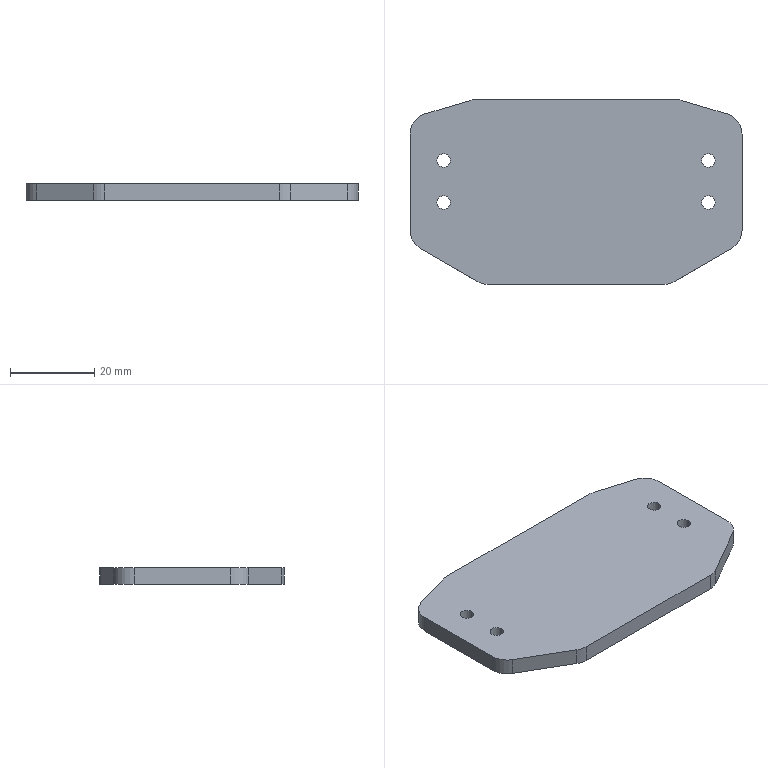Part | SolidWorks | features Extrusion 1, Fillet 1 | 1 solid | 26 faces | box 79 x 44 x 4 mm | volume 12779 mm3 | cylinder 16 | plane 10 | commonest cylinder face diameters 3.2 x8 10 x8
STEP:
#1=CARTESIAN_POINT('',(29.9,9.,4.));
#2=VERTEX_POINT('',#1);
#3=CARTESIAN_POINT('',(33.1,9.,4.));
#4=VERTEX_POINT('',#3);
#5=CARTESIAN_POINT('',(31.5,9.,4.));
#6=DIRECTION('',(0.,0.,1.));
#7=DIRECTION('',(-1.,0.,0.));
#8=AXIS2_PLACEMENT_3D('',#5,#6,#7);
#9=CIRCLE('',#8,1.6);
#10=EDGE_CURVE('',#2,#4,#9,.T.);
#11=ORIENTED_EDGE('',*,*,#10,.T.);
#12=CARTESIAN_POINT('',(33.1,9.,0.));
#13=VERTEX_POINT('',#12);
#14=CARTESIAN_POINT('',(33.1,9.,4.));
#15=DIRECTION('',(0.,0.,-1.));
#16=VECTOR('',#15,1000.);
#17=LINE('',#14,#16);
#18=EDGE_CURVE('',#4,#13,#17,.T.);
#19=ORIENTED_EDGE('',*,*,#18,.T.);
#20=CARTESIAN_POINT('',(29.9,9.,0.));
#21=VERTEX_POINT('',#20);
#22=CARTESIAN_POINT('',(31.5,9.,0.));
#23=DIRECTION('',(0.,0.,1.));
#24=DIRECTION('',(-1.,0.,0.));
#25=AXIS2_PLACEMENT_3D('',#22,#23,#24);
#26=CIRCLE('',#25,1.6);
#27=EDGE_CURVE('',#21,#13,#26,.T.);
#28=ORIENTED_EDGE('',*,*,#27,.F.);
#29=CARTESIAN_POINT('',(29.9,9.,4.));
#30=DIRECTION('',(0.,0.,-1.));
#31=VECTOR('',#30,1000.);
#32=LINE('',#29,#31);
#33=EDGE_CURVE('',#2,#21,#32,.T.);
#34=ORIENTED_EDGE('',*,*,#33,.F.);
#35=EDGE_LOOP('',(#11,#19,#28,#34));
#36=FACE_OUTER_BOUND('',#35,.T.);
#37=CARTESIAN_POINT('',(31.5,9.,4.));
#38=DIRECTION('',(0.,0.,-1.));
#39=DIRECTION('',(-1.,0.,0.));
#40=AXIS2_PLACEMENT_3D('',#37,#38,#39);
#41=CYLINDRICAL_SURFACE('',#40,1.6);
#42=ADVANCED_FACE('',(#36),#41,.F.);
#43=CARTESIAN_POINT('',(29.9,-1.,4.));
#44=VERTEX_POINT('',#43);
#45=CARTESIAN_POINT('',(33.1,-1.,4.));
#46=VERTEX_POINT('',#45);
#47=CARTESIAN_POINT('',(31.5,-1.,4.));
#48=DIRECTION('',(0.,0.,1.));
#49=DIRECTION('',(-1.,0.,0.));
#50=AXIS2_PLACEMENT_3D('',#47,#48,#49);
#51=CIRCLE('',#50,1.6);
#52=EDGE_CURVE('',#44,#46,#51,.T.);
#53=ORIENTED_EDGE('',*,*,#52,.T.);
#54=CARTESIAN_POINT('',(33.1,-1.,0.));
#55=VERTEX_POINT('',#54);
#56=CARTESIAN_POINT('',(33.1,-1.,4.));
#57=DIRECTION('',(0.,0.,-1.));
#58=VECTOR('',#57,1000.);
#59=LINE('',#56,#58);
#60=EDGE_CURVE('',#46,#55,#59,.T.);
#61=ORIENTED_EDGE('',*,*,#60,.T.);
#62=CARTESIAN_POINT('',(29.9,-1.,0.));
#63=VERTEX_POINT('',#62);
#64=CARTESIAN_POINT('',(31.5,-1.,0.));
#65=DIRECTION('',(0.,0.,1.));
#66=DIRECTION('',(-1.,0.,0.));
#67=AXIS2_PLACEMENT_3D('',#64,#65,#66);
#68=CIRCLE('',#67,1.6);
#69=EDGE_CURVE('',#63,#55,#68,.T.);
#70=ORIENTED_EDGE('',*,*,#69,.F.);
#71=CARTESIAN_POINT('',(29.9,-1.,4.));
#72=DIRECTION('',(0.,0.,-1.));
#73=VECTOR('',#72,1000.);
#74=LINE('',#71,#73);
#75=EDGE_CURVE('',#44,#63,#74,.T.);
#76=ORIENTED_EDGE('',*,*,#75,.F.);
#77=EDGE_LOOP('',(#53,#61,#70,#76));
#78=FACE_OUTER_BOUND('',#77,.T.);
#79=CARTESIAN_POINT('',(31.5,-1.,4.));
#80=DIRECTION('',(0.,0.,-1.));
#81=DIRECTION('',(-1.,0.,0.));
#82=AXIS2_PLACEMENT_3D('',#79,#80,#81);
#83=CYLINDRICAL_SURFACE('',#82,1.6);
#84=ADVANCED_FACE('',(#78),#83,.F.);
#85=CARTESIAN_POINT('',(-33.1,-1.,4.));
#86=VERTEX_POINT('',#85);
#87=CARTESIAN_POINT('',(-29.9,-1.,4.));
#88=VERTEX_POINT('',#87);
#89=CARTESIAN_POINT('',(-31.5,-1.,4.));
#90=DIRECTION('',(0.,0.,1.));
#91=DIRECTION('',(1.,0.,0.));
#92=AXIS2_PLACEMENT_3D('',#89,#90,#91);
#93=CIRCLE('',#92,1.6);
#94=EDGE_CURVE('',#86,#88,#93,.T.);
#95=ORIENTED_EDGE('',*,*,#94,.T.);
#96=CARTESIAN_POINT('',(-29.9,-1.,0.));
#97=VERTEX_POINT('',#96);
#98=CARTESIAN_POINT('',(-29.9,-1.,4.));
#99=DIRECTION('',(0.,0.,-1.));
#100=VECTOR('',#99,1000.);
#101=LINE('',#98,#100);
#102=EDGE_CURVE('',#88,#97,#101,.T.);
#103=ORIENTED_EDGE('',*,*,#102,.T.);
#104=CARTESIAN_POINT('',(-33.1,-1.,0.));
#105=VERTEX_POINT('',#104);
#106=CARTESIAN_POINT('',(-31.5,-1.,0.));
#107=DIRECTION('',(0.,0.,1.));
#108=DIRECTION('',(1.,0.,0.));
#109=AXIS2_PLACEMENT_3D('',#106,#107,#108);
#110=CIRCLE('',#109,1.6);
#111=EDGE_CURVE('',#105,#97,#110,.T.);
#112=ORIENTED_EDGE('',*,*,#111,.F.);
#113=CARTESIAN_POINT('',(-33.1,-1.,4.));
#114=DIRECTION('',(0.,0.,-1.));
#115=VECTOR('',#114,1000.);
#116=LINE('',#113,#115);
#117=EDGE_CURVE('',#86,#105,#116,.T.);
#118=ORIENTED_EDGE('',*,*,#117,.F.);
#119=EDGE_LOOP('',(#95,#103,#112,#118));
#120=FACE_OUTER_BOUND('',#119,.T.);
#121=CARTESIAN_POINT('',(-31.5,-1.,4.));
#122=DIRECTION('',(0.,0.,-1.));
#123=DIRECTION('',(-1.,0.,0.));
#124=AXIS2_PLACEMENT_3D('',#121,#122,#123);
#125=CYLINDRICAL_SURFACE('',#124,1.6);
#126=ADVANCED_FACE('',(#120),#125,.F.);
#127=CARTESIAN_POINT('',(-33.1,9.,4.));
#128=VERTEX_POINT('',#127);
#129=CARTESIAN_POINT('',(-29.9,9.,4.));
#130=VERTEX_POINT('',#129);
#131=CARTESIAN_POINT('',(-31.5,9.,4.));
#132=DIRECTION('',(0.,0.,1.));
#133=DIRECTION('',(1.,0.,0.));
#134=AXIS2_PLACEMENT_3D('',#131,#132,#133);
#135=CIRCLE('',#134,1.6);
#136=EDGE_CURVE('',#128,#130,#135,.T.);
#137=ORIENTED_EDGE('',*,*,#136,.T.);
#138=CARTESIAN_POINT('',(-29.9,9.,0.));
#139=VERTEX_POINT('',#138);
#140=CARTESIAN_POINT('',(-29.9,9.,4.));
#141=DIRECTION('',(0.,0.,-1.));
#142=VECTOR('',#141,1000.);
#143=LINE('',#140,#142);
#144=EDGE_CURVE('',#130,#139,#143,.T.);
#145=ORIENTED_EDGE('',*,*,#144,.T.);
#146=CARTESIAN_POINT('',(-33.1,9.,0.));
#147=VERTEX_POINT('',#146);
#148=CARTESIAN_POINT('',(-31.5,9.,0.));
#149=DIRECTION('',(0.,0.,1.));
#150=DIRECTION('',(1.,0.,0.));
#151=AXIS2_PLACEMENT_3D('',#148,#149,#150);
#152=CIRCLE('',#151,1.6);
#153=EDGE_CURVE('',#147,#139,#152,.T.);
#154=ORIENTED_EDGE('',*,*,#153,.F.);
#155=CARTESIAN_POINT('',(-33.1,9.,4.));
#156=DIRECTION('',(0.,0.,-1.));
#157=VECTOR('',#156,1000.);
#158=LINE('',#155,#157);
#159=EDGE_CURVE('',#128,#147,#158,.T.);
#160=ORIENTED_EDGE('',*,*,#159,.F.);
#161=EDGE_LOOP('',(#137,#145,#154,#160));
#162=FACE_OUTER_BOUND('',#161,.T.);
#163=CARTESIAN_POINT('',(-31.5,9.,4.));
#164=DIRECTION('',(0.,0.,-1.));
#165=DIRECTION('',(-1.,0.,0.));
#166=AXIS2_PLACEMENT_3D('',#163,#164,#165);
#167=CYLINDRICAL_SURFACE('',#166,1.6);
#168=ADVANCED_FACE('',(#162),#167,.F.);
#169=CARTESIAN_POINT('',(-39.5,15.28,4.));
#170=VERTEX_POINT('',#169);
#171=CARTESIAN_POINT('',(-39.5,-7.613,4.));
#172=VERTEX_POINT('',#171);
#173=CARTESIAN_POINT('',(-39.5,19.,4.));
#174=DIRECTION('',(0.,-1.,0.));
#175=VECTOR('',#174,1000.);
#176=LINE('',#173,#175);
#177=EDGE_CURVE('',#170,#172,#176,.T.);
#178=ORIENTED_EDGE('',*,*,#177,.T.);
#179=CARTESIAN_POINT('',(-37.,-11.943,4.));
#180=VERTEX_POINT('',#179);
#181=CARTESIAN_POINT('',(-34.5,-7.613,4.));
#182=DIRECTION('',(0.,0.,1.));
#183=DIRECTION('',(-1.,0.,0.));
#184=AXIS2_PLACEMENT_3D('',#181,#182,#183);
#185=CIRCLE('',#184,5.);
#186=EDGE_CURVE('',#172,#180,#185,.T.);
#187=ORIENTED_EDGE('',*,*,#186,.T.);
#188=CARTESIAN_POINT('',(-23.34,-19.83,4.));
#189=VERTEX_POINT('',#188);
#190=CARTESIAN_POINT('',(-39.5,-10.5,4.));
#191=DIRECTION('',(0.866,-0.5,0.));
#192=VECTOR('',#191,1000.);
#193=LINE('',#190,#192);
#194=EDGE_CURVE('',#180,#189,#193,.T.);
#195=ORIENTED_EDGE('',*,*,#194,.T.);
#196=CARTESIAN_POINT('',(-20.84,-20.5,4.));
#197=VERTEX_POINT('',#196);
#198=CARTESIAN_POINT('',(-20.84,-15.5,4.));
#199=DIRECTION('',(0.,0.,1.));
#200=DIRECTION('',(-1.,0.,0.));
#201=AXIS2_PLACEMENT_3D('',#198,#199,#200);
#202=CIRCLE('',#201,5.);
#203=EDGE_CURVE('',#189,#197,#202,.T.);
#204=ORIENTED_EDGE('',*,*,#203,.T.);
#205=CARTESIAN_POINT('',(20.84,-20.5,4.));
#206=VERTEX_POINT('',#205);
#207=CARTESIAN_POINT('',(-22.179,-20.5,4.));
#208=DIRECTION('',(1.,0.,0.));
#209=VECTOR('',#208,1000.);
#210=LINE('',#207,#209);
#211=EDGE_CURVE('',#197,#206,#210,.T.);
#212=ORIENTED_EDGE('',*,*,#211,.T.);
#213=CARTESIAN_POINT('',(23.34,-19.83,4.));
#214=VERTEX_POINT('',#213);
#215=CARTESIAN_POINT('',(20.84,-15.5,4.));
#216=DIRECTION('',(0.,0.,1.));
#217=DIRECTION('',(-1.,0.,0.));
#218=AXIS2_PLACEMENT_3D('',#215,#216,#217);
#219=CIRCLE('',#218,5.);
#220=EDGE_CURVE('',#206,#214,#219,.T.);
#221=ORIENTED_EDGE('',*,*,#220,.T.);
#222=CARTESIAN_POINT('',(37.,-11.943,4.));
#223=VERTEX_POINT('',#222);
#224=CARTESIAN_POINT('',(39.5,-10.5,4.));
#225=DIRECTION('',(0.866,0.5,0.));
#226=VECTOR('',#225,1000.);
#227=LINE('',#224,#226);
#228=EDGE_CURVE('',#214,#223,#227,.T.);
#229=ORIENTED_EDGE('',*,*,#228,.T.);
#230=CARTESIAN_POINT('',(39.5,-7.613,4.));
#231=VERTEX_POINT('',#230);
#232=CARTESIAN_POINT('',(34.5,-7.613,4.));
#233=DIRECTION('',(0.,0.,1.));
#234=DIRECTION('',(-1.,0.,0.));
#235=AXIS2_PLACEMENT_3D('',#232,#233,#234);
#236=CIRCLE('',#235,5.);
#237=EDGE_CURVE('',#223,#231,#236,.T.);
#238=ORIENTED_EDGE('',*,*,#237,.T.);
#239=CARTESIAN_POINT('',(39.5,15.28,4.));
#240=VERTEX_POINT('',#239);
#241=CARTESIAN_POINT('',(39.5,19.,4.));
#242=DIRECTION('',(0.,1.,0.));
#243=VECTOR('',#242,1000.);
#244=LINE('',#241,#243);
#245=EDGE_CURVE('',#231,#240,#244,.T.);
#246=ORIENTED_EDGE('',*,*,#245,.T.);
#247=CARTESIAN_POINT('',(35.937,20.069,4.));
#248=VERTEX_POINT('',#247);
#249=CARTESIAN_POINT('',(34.5,15.28,4.));
#250=DIRECTION('',(0.,0.,1.));
#251=DIRECTION('',(-1.,0.,0.));
#252=AXIS2_PLACEMENT_3D('',#249,#250,#251);
#253=CIRCLE('',#252,5.);
#254=EDGE_CURVE('',#240,#248,#253,.T.);
#255=ORIENTED_EDGE('',*,*,#254,.T.);
#256=CARTESIAN_POINT('',(25.203,23.289,4.));
#257=VERTEX_POINT('',#256);
#258=CARTESIAN_POINT('',(39.5,19.,4.));
#259=DIRECTION('',(-0.9578,0.2873,0.));
#260=VECTOR('',#259,1000.);
#261=LINE('',#258,#260);
#262=EDGE_CURVE('',#248,#257,#261,.T.);
#263=ORIENTED_EDGE('',*,*,#262,.T.);
#264=CARTESIAN_POINT('',(23.766,23.5,4.));
#265=VERTEX_POINT('',#264);
#266=CARTESIAN_POINT('',(23.766,18.5,4.));
#267=DIRECTION('',(0.,0.,1.));
#268=DIRECTION('',(-1.,0.,0.));
#269=AXIS2_PLACEMENT_3D('',#266,#267,#268);
#270=CIRCLE('',#269,5.);
#271=EDGE_CURVE('',#257,#265,#270,.T.);
#272=ORIENTED_EDGE('',*,*,#271,.T.);
#273=CARTESIAN_POINT('',(-23.766,23.5,4.));
#274=VERTEX_POINT('',#273);
#275=CARTESIAN_POINT('',(-24.5,23.5,4.));
#276=DIRECTION('',(-1.,0.,0.));
#277=VECTOR('',#276,1000.);
#278=LINE('',#275,#277);
#279=EDGE_CURVE('',#265,#274,#278,.T.);
#280=ORIENTED_EDGE('',*,*,#279,.T.);
#281=CARTESIAN_POINT('',(-25.203,23.289,4.));
#282=VERTEX_POINT('',#281);
#283=CARTESIAN_POINT('',(-23.766,18.5,4.));
#284=DIRECTION('',(0.,0.,1.));
#285=DIRECTION('',(-1.,0.,0.));
#286=AXIS2_PLACEMENT_3D('',#283,#284,#285);
#287=CIRCLE('',#286,5.);
#288=EDGE_CURVE('',#274,#282,#287,.T.);
#289=ORIENTED_EDGE('',*,*,#288,.T.);
#290=CARTESIAN_POINT('',(-35.937,20.069,4.));
#291=VERTEX_POINT('',#290);
#292=CARTESIAN_POINT('',(-39.5,19.,4.));
#293=DIRECTION('',(-0.9578,-0.2873,0.));
#294=VECTOR('',#293,1000.);
#295=LINE('',#292,#294);
#296=EDGE_CURVE('',#282,#291,#295,.T.);
#297=ORIENTED_EDGE('',*,*,#296,.T.);
#298=CARTESIAN_POINT('',(-34.5,15.28,4.));
#299=DIRECTION('',(0.,0.,1.));
#300=DIRECTION('',(-1.,0.,0.));
#301=AXIS2_PLACEMENT_3D('',#298,#299,#300);
#302=CIRCLE('',#301,5.);
#303=EDGE_CURVE('',#291,#170,#302,.T.);
#304=ORIENTED_EDGE('',*,*,#303,.T.);
#305=EDGE_LOOP('',(#178,#187,#195,#204,#212,#221,#229,#238,#246,#255,#263,#272,#280,#289,#297,#304));
#306=FACE_OUTER_BOUND('',#305,.T.);
#307=ORIENTED_EDGE('',*,*,#136,.F.);
#308=CARTESIAN_POINT('',(-31.5,9.,4.));
#309=DIRECTION('',(0.,0.,1.));
#310=DIRECTION('',(1.,0.,0.));
#311=AXIS2_PLACEMENT_3D('',#308,#309,#310);
#312=CIRCLE('',#311,1.6);
#313=EDGE_CURVE('',#130,#128,#312,.T.);
#314=ORIENTED_EDGE('',*,*,#313,.F.);
#315=EDGE_LOOP('',(#307,#314));
#316=FACE_BOUND('',#315,.T.);
#317=ORIENTED_EDGE('',*,*,#94,.F.);
#318=CARTESIAN_POINT('',(-31.5,-1.,4.));
#319=DIRECTION('',(0.,0.,1.));
#320=DIRECTION('',(1.,0.,0.));
#321=AXIS2_PLACEMENT_3D('',#318,#319,#320);
#322=CIRCLE('',#321,1.6);
#323=EDGE_CURVE('',#88,#86,#322,.T.);
#324=ORIENTED_EDGE('',*,*,#323,.F.);
#325=EDGE_LOOP('',(#317,#324));
#326=FACE_BOUND('',#325,.T.);
#327=ORIENTED_EDGE('',*,*,#52,.F.);
#328=CARTESIAN_POINT('',(31.5,-1.,4.));
#329=DIRECTION('',(0.,0.,1.));
#330=DIRECTION('',(-1.,0.,0.));
#331=AXIS2_PLACEMENT_3D('',#328,#329,#330);
#332=CIRCLE('',#331,1.6);
#333=EDGE_CURVE('',#46,#44,#332,.T.);
#334=ORIENTED_EDGE('',*,*,#333,.F.);
#335=EDGE_LOOP('',(#327,#334));
#336=FACE_BOUND('',#335,.T.);
#337=ORIENTED_EDGE('',*,*,#10,.F.);
#338=CARTESIAN_POINT('',(31.5,9.,4.));
#339=DIRECTION('',(0.,0.,1.));
#340=DIRECTION('',(-1.,0.,0.));
#341=AXIS2_PLACEMENT_3D('',#338,#339,#340);
#342=CIRCLE('',#341,1.6);
#343=EDGE_CURVE('',#4,#2,#342,.T.);
#344=ORIENTED_EDGE('',*,*,#343,.F.);
#345=EDGE_LOOP('',(#337,#344));
#346=FACE_BOUND('',#345,.T.);
#347=CARTESIAN_POINT('',(0.,0.,4.));
#348=DIRECTION('',(0.,0.,-1.));
#349=DIRECTION('',(-1.,0.,0.));
#350=AXIS2_PLACEMENT_3D('',#347,#348,#349);
#351=PLANE('',#350);
#352=ADVANCED_FACE('',(#306,#316,#326,#336,#346),#351,.F.);
#353=ORIENTED_EDGE('',*,*,#69,.T.);
#354=CARTESIAN_POINT('',(31.5,-1.,0.));
#355=DIRECTION('',(0.,0.,1.));
#356=DIRECTION('',(-1.,0.,0.));
#357=AXIS2_PLACEMENT_3D('',#354,#355,#356);
#358=CIRCLE('',#357,1.6);
#359=EDGE_CURVE('',#55,#63,#358,.T.);
#360=ORIENTED_EDGE('',*,*,#359,.T.);
#361=EDGE_LOOP('',(#353,#360));
#362=FACE_BOUND('',#361,.T.);
#363=ORIENTED_EDGE('',*,*,#153,.T.);
#364=CARTESIAN_POINT('',(-31.5,9.,0.));
#365=DIRECTION('',(0.,0.,1.));
#366=DIRECTION('',(1.,0.,0.));
#367=AXIS2_PLACEMENT_3D('',#364,#365,#366);
#368=CIRCLE('',#367,1.6);
#369=EDGE_CURVE('',#139,#147,#368,.T.);
#370=ORIENTED_EDGE('',*,*,#369,.T.);
#371=EDGE_LOOP('',(#363,#370));
#372=FACE_BOUND('',#371,.T.);
#373=CARTESIAN_POINT('',(-37.,-11.943,0.));
#374=VERTEX_POINT('',#373);
#375=CARTESIAN_POINT('',(-23.34,-19.83,0.));
#376=VERTEX_POINT('',#375);
#377=CARTESIAN_POINT('',(-39.5,-10.5,0.));
#378=DIRECTION('',(0.866,-0.5,0.));
#379=VECTOR('',#378,1000.);
#380=LINE('',#377,#379);
#381=EDGE_CURVE('',#374,#376,#380,.T.);
#382=ORIENTED_EDGE('',*,*,#381,.F.);
#383=CARTESIAN_POINT('',(-39.5,-7.613,0.));
#384=VERTEX_POINT('',#383);
#385=CARTESIAN_POINT('',(-34.5,-7.613,0.));
#386=DIRECTION('',(0.,0.,-1.));
#387=DIRECTION('',(-1.,0.,0.));
#388=AXIS2_PLACEMENT_3D('',#385,#386,#387);
#389=CIRCLE('',#388,5.);
#390=EDGE_CURVE('',#374,#384,#389,.T.);
#391=ORIENTED_EDGE('',*,*,#390,.T.);
#392=CARTESIAN_POINT('',(-39.5,15.28,0.));
#393=VERTEX_POINT('',#392);
#394=CARTESIAN_POINT('',(-39.5,19.,0.));
#395=DIRECTION('',(0.,-1.,0.));
#396=VECTOR('',#395,1000.);
#397=LINE('',#394,#396);
#398=EDGE_CURVE('',#393,#384,#397,.T.);
#399=ORIENTED_EDGE('',*,*,#398,.F.);
#400=CARTESIAN_POINT('',(-35.937,20.069,0.));
#401=VERTEX_POINT('',#400);
#402=CARTESIAN_POINT('',(-34.5,15.28,0.));
#403=DIRECTION('',(0.,0.,-1.));
#404=DIRECTION('',(-1.,0.,0.));
#405=AXIS2_PLACEMENT_3D('',#402,#403,#404);
#406=CIRCLE('',#405,5.);
#407=EDGE_CURVE('',#393,#401,#406,.T.);
#408=ORIENTED_EDGE('',*,*,#407,.T.);
#409=CARTESIAN_POINT('',(-25.203,23.289,0.));
#410=VERTEX_POINT('',#409);
#411=CARTESIAN_POINT('',(-39.5,19.,0.));
#412=DIRECTION('',(-0.9578,-0.2873,0.));
#413=VECTOR('',#412,1000.);
#414=LINE('',#411,#413);
#415=EDGE_CURVE('',#410,#401,#414,.T.);
#416=ORIENTED_EDGE('',*,*,#415,.F.);
#417=CARTESIAN_POINT('',(-23.766,23.5,0.));
#418=VERTEX_POINT('',#417);
#419=CARTESIAN_POINT('',(-23.766,18.5,0.));
#420=DIRECTION('',(0.,0.,-1.));
#421=DIRECTION('',(-1.,0.,0.));
#422=AXIS2_PLACEMENT_3D('',#419,#420,#421);
#423=CIRCLE('',#422,5.);
#424=EDGE_CURVE('',#410,#418,#423,.T.);
#425=ORIENTED_EDGE('',*,*,#424,.T.);
#426=CARTESIAN_POINT('',(23.766,23.5,0.));
#427=VERTEX_POINT('',#426);
#428=CARTESIAN_POINT('',(-24.5,23.5,0.));
#429=DIRECTION('',(-1.,0.,0.));
#430=VECTOR('',#429,1000.);
#431=LINE('',#428,#430);
#432=EDGE_CURVE('',#427,#418,#431,.T.);
#433=ORIENTED_EDGE('',*,*,#432,.F.);
#434=CARTESIAN_POINT('',(25.203,23.289,0.));
#435=VERTEX_POINT('',#434);
#436=CARTESIAN_POINT('',(23.766,18.5,0.));
#437=DIRECTION('',(0.,0.,-1.));
#438=DIRECTION('',(-1.,0.,0.));
#439=AXIS2_PLACEMENT_3D('',#436,#437,#438);
#440=CIRCLE('',#439,5.);
#441=EDGE_CURVE('',#427,#435,#440,.T.);
#442=ORIENTED_EDGE('',*,*,#441,.T.);
#443=CARTESIAN_POINT('',(35.937,20.069,0.));
#444=VERTEX_POINT('',#443);
#445=CARTESIAN_POINT('',(39.5,19.,0.));
#446=DIRECTION('',(-0.9578,0.2873,0.));
#447=VECTOR('',#446,1000.);
#448=LINE('',#445,#447);
#449=EDGE_CURVE('',#444,#435,#448,.T.);
#450=ORIENTED_EDGE('',*,*,#449,.F.);
#451=CARTESIAN_POINT('',(39.5,15.28,0.));
#452=VERTEX_POINT('',#451);
#453=CARTESIAN_POINT('',(34.5,15.28,0.));
#454=DIRECTION('',(0.,0.,-1.));
#455=DIRECTION('',(-1.,0.,0.));
#456=AXIS2_PLACEMENT_3D('',#453,#454,#455);
#457=CIRCLE('',#456,5.);
#458=EDGE_CURVE('',#444,#452,#457,.T.);
#459=ORIENTED_EDGE('',*,*,#458,.T.);
#460=CARTESIAN_POINT('',(39.5,-7.613,0.));
#461=VERTEX_POINT('',#460);
#462=CARTESIAN_POINT('',(39.5,19.,0.));
#463=DIRECTION('',(0.,1.,0.));
#464=VECTOR('',#463,1000.);
#465=LINE('',#462,#464);
#466=EDGE_CURVE('',#461,#452,#465,.T.);
#467=ORIENTED_EDGE('',*,*,#466,.F.);
#468=CARTESIAN_POINT('',(37.,-11.943,0.));
#469=VERTEX_POINT('',#468);
#470=CARTESIAN_POINT('',(34.5,-7.613,0.));
#471=DIRECTION('',(0.,0.,-1.));
#472=DIRECTION('',(-1.,0.,0.));
#473=AXIS2_PLACEMENT_3D('',#470,#471,#472);
#474=CIRCLE('',#473,5.);
#475=EDGE_CURVE('',#461,#469,#474,.T.);
#476=ORIENTED_EDGE('',*,*,#475,.T.);
#477=CARTESIAN_POINT('',(23.34,-19.83,0.));
#478=VERTEX_POINT('',#477);
#479=CARTESIAN_POINT('',(39.5,-10.5,0.));
#480=DIRECTION('',(0.866,0.5,0.));
#481=VECTOR('',#480,1000.);
#482=LINE('',#479,#481);
#483=EDGE_CURVE('',#478,#469,#482,.T.);
#484=ORIENTED_EDGE('',*,*,#483,.F.);
#485=CARTESIAN_POINT('',(20.84,-20.5,0.));
#486=VERTEX_POINT('',#485);
#487=CARTESIAN_POINT('',(20.84,-15.5,0.));
#488=DIRECTION('',(0.,0.,-1.));
#489=DIRECTION('',(-1.,0.,0.));
#490=AXIS2_PLACEMENT_3D('',#487,#488,#489);
#491=CIRCLE('',#490,5.);
#492=EDGE_CURVE('',#478,#486,#491,.T.);
#493=ORIENTED_EDGE('',*,*,#492,.T.);
#494=CARTESIAN_POINT('',(-20.84,-20.5,0.));
#495=VERTEX_POINT('',#494);
#496=CARTESIAN_POINT('',(-22.179,-20.5,0.));
#497=DIRECTION('',(1.,0.,0.));
#498=VECTOR('',#497,1000.);
#499=LINE('',#496,#498);
#500=EDGE_CURVE('',#495,#486,#499,.T.);
#501=ORIENTED_EDGE('',*,*,#500,.F.);
#502=CARTESIAN_POINT('',(-20.84,-15.5,0.));
#503=DIRECTION('',(0.,0.,-1.));
#504=DIRECTION('',(-1.,0.,0.));
#505=AXIS2_PLACEMENT_3D('',#502,#503,#504);
#506=CIRCLE('',#505,5.);
#507=EDGE_CURVE('',#495,#376,#506,.T.);
#508=ORIENTED_EDGE('',*,*,#507,.T.);
#509=EDGE_LOOP('',(#382,#391,#399,#408,#416,#425,#433,#442,#450,#459,#467,#476,#484,#493,#501,#508));
#510=FACE_OUTER_BOUND('',#509,.T.);
#511=ORIENTED_EDGE('',*,*,#111,.T.);
#512=CARTESIAN_POINT('',(-31.5,-1.,0.));
#513=DIRECTION('',(0.,0.,1.));
#514=DIRECTION('',(1.,0.,0.));
#515=AXIS2_PLACEMENT_3D('',#512,#513,#514);
#516=CIRCLE('',#515,1.6);
#517=EDGE_CURVE('',#97,#105,#516,.T.);
#518=ORIENTED_EDGE('',*,*,#517,.T.);
#519=EDGE_LOOP('',(#511,#518));
#520=FACE_BOUND('',#519,.T.);
#521=ORIENTED_EDGE('',*,*,#27,.T.);
#522=CARTESIAN_POINT('',(31.5,9.,0.));
#523=DIRECTION('',(0.,0.,1.));
#524=DIRECTION('',(-1.,0.,0.));
#525=AXIS2_PLACEMENT_3D('',#522,#523,#524);
#526=CIRCLE('',#525,1.6);
#527=EDGE_CURVE('',#13,#21,#526,.T.);
#528=ORIENTED_EDGE('',*,*,#527,.T.);
#529=EDGE_LOOP('',(#521,#528));
#530=FACE_BOUND('',#529,.T.);
#531=CARTESIAN_POINT('',(0.,0.,0.));
#532=DIRECTION('',(0.,0.,-1.));
#533=DIRECTION('',(-1.,0.,0.));
#534=AXIS2_PLACEMENT_3D('',#531,#532,#533);
#535=PLANE('',#534);
#536=ADVANCED_FACE('',(#362,#372,#510,#520,#530),#535,.T.);
#537=ORIENTED_EDGE('',*,*,#296,.F.);
#538=CARTESIAN_POINT('',(-25.203,23.289,4.));
#539=DIRECTION('',(0.,0.,-1.));
#540=VECTOR('',#539,1000.);
#541=LINE('',#538,#540);
#542=EDGE_CURVE('',#282,#410,#541,.T.);
#543=ORIENTED_EDGE('',*,*,#542,.T.);
#544=ORIENTED_EDGE('',*,*,#415,.T.);
#545=CARTESIAN_POINT('',(-35.937,20.069,4.));
#546=DIRECTION('',(0.,0.,1.));
#547=VECTOR('',#546,1000.);
#548=LINE('',#545,#547);
#549=EDGE_CURVE('',#401,#291,#548,.T.);
#550=ORIENTED_EDGE('',*,*,#549,.T.);
#551=EDGE_LOOP('',(#537,#543,#544,#550));
#552=FACE_OUTER_BOUND('',#551,.T.);
#553=CARTESIAN_POINT('',(-39.5,19.,4.));
#554=DIRECTION('',(0.2873,-0.9578,0.));
#555=DIRECTION('',(0.9578,0.2873,0.));
#556=AXIS2_PLACEMENT_3D('',#553,#554,#555);
#557=PLANE('',#556);
#558=ADVANCED_FACE('',(#552),#557,.F.);
#559=ORIENTED_EDGE('',*,*,#398,.T.);
#560=CARTESIAN_POINT('',(-39.5,-7.613,4.));
#561=DIRECTION('',(0.,0.,1.));
#562=VECTOR('',#561,1000.);
#563=LINE('',#560,#562);
#564=EDGE_CURVE('',#384,#172,#563,.T.);
#565=ORIENTED_EDGE('',*,*,#564,.T.);
#566=ORIENTED_EDGE('',*,*,#177,.F.);
#567=CARTESIAN_POINT('',(-39.5,15.28,4.));
#568=DIRECTION('',(0.,0.,-1.));
#569=VECTOR('',#568,1000.);
#570=LINE('',#567,#569);
#571=EDGE_CURVE('',#170,#393,#570,.T.);
#572=ORIENTED_EDGE('',*,*,#571,.T.);
#573=EDGE_LOOP('',(#559,#565,#566,#572));
#574=FACE_OUTER_BOUND('',#573,.T.);
#575=CARTESIAN_POINT('',(-39.5,19.,4.));
#576=DIRECTION('',(1.,0.,0.));
#577=DIRECTION('',(0.,1.,0.));
#578=AXIS2_PLACEMENT_3D('',#575,#576,#577);
#579=PLANE('',#578);
#580=ADVANCED_FACE('',(#574),#579,.F.);
#581=ORIENTED_EDGE('',*,*,#194,.F.);
#582=CARTESIAN_POINT('',(-37.,-11.943,4.));
#583=DIRECTION('',(0.,0.,-1.));
#584=VECTOR('',#583,1000.);
#585=LINE('',#582,#584);
#586=EDGE_CURVE('',#180,#374,#585,.T.);
#587=ORIENTED_EDGE('',*,*,#586,.T.);
#588=ORIENTED_EDGE('',*,*,#381,.T.);
#589=CARTESIAN_POINT('',(-23.34,-19.83,4.));
#590=DIRECTION('',(0.,0.,1.));
#591=VECTOR('',#590,1000.);
#592=LINE('',#589,#591);
#593=EDGE_CURVE('',#376,#189,#592,.T.);
#594=ORIENTED_EDGE('',*,*,#593,.T.);
#595=EDGE_LOOP('',(#581,#587,#588,#594));
#596=FACE_OUTER_BOUND('',#595,.T.);
#597=CARTESIAN_POINT('',(-39.5,-10.5,4.));
#598=DIRECTION('',(0.5,0.866,0.));
#599=DIRECTION('',(-0.866,0.5,0.));
#600=AXIS2_PLACEMENT_3D('',#597,#598,#599);
#601=PLANE('',#600);
#602=ADVANCED_FACE('',(#596),#601,.F.);
#603=ORIENTED_EDGE('',*,*,#211,.F.);
#604=CARTESIAN_POINT('',(-20.84,-20.5,4.));
#605=DIRECTION('',(0.,0.,-1.));
#606=VECTOR('',#605,1000.);
#607=LINE('',#604,#606);
#608=EDGE_CURVE('',#197,#495,#607,.T.);
#609=ORIENTED_EDGE('',*,*,#608,.T.);
#610=ORIENTED_EDGE('',*,*,#500,.T.);
#611=CARTESIAN_POINT('',(20.84,-20.5,4.));
#612=DIRECTION('',(0.,0.,1.));
#613=VECTOR('',#612,1000.);
#614=LINE('',#611,#613);
#615=EDGE_CURVE('',#486,#206,#614,.T.);
#616=ORIENTED_EDGE('',*,*,#615,.T.);
#617=EDGE_LOOP('',(#603,#609,#610,#616));
#618=FACE_OUTER_BOUND('',#617,.T.);
#619=CARTESIAN_POINT('',(-22.179,-20.5,4.));
#620=DIRECTION('',(0.,1.,0.));
#621=DIRECTION('',(-1.,0.,0.));
#622=AXIS2_PLACEMENT_3D('',#619,#620,#621);
#623=PLANE('',#622);
#624=ADVANCED_FACE('',(#618),#623,.F.);
#625=ORIENTED_EDGE('',*,*,#228,.F.);
#626=CARTESIAN_POINT('',(23.34,-19.83,4.));
#627=DIRECTION('',(0.,0.,-1.));
#628=VECTOR('',#627,1000.);
#629=LINE('',#626,#628);
#630=EDGE_CURVE('',#214,#478,#629,.T.);
#631=ORIENTED_EDGE('',*,*,#630,.T.);
#632=ORIENTED_EDGE('',*,*,#483,.T.);
#633=CARTESIAN_POINT('',(37.,-11.943,4.));
#634=DIRECTION('',(0.,0.,1.));
#635=VECTOR('',#634,1000.);
#636=LINE('',#633,#635);
#637=EDGE_CURVE('',#469,#223,#636,.T.);
#638=ORIENTED_EDGE('',*,*,#637,.T.);
#639=EDGE_LOOP('',(#625,#631,#632,#638));
#640=FACE_OUTER_BOUND('',#639,.T.);
#641=CARTESIAN_POINT('',(39.5,-10.5,4.));
#642=DIRECTION('',(-0.5,0.866,0.));
#643=DIRECTION('',(-0.866,-0.5,0.));
#644=AXIS2_PLACEMENT_3D('',#641,#642,#643);
#645=PLANE('',#644);
#646=ADVANCED_FACE('',(#640),#645,.F.);
#647=ORIENTED_EDGE('',*,*,#245,.F.);
#648=CARTESIAN_POINT('',(39.5,-7.613,4.));
#649=DIRECTION('',(0.,0.,-1.));
#650=VECTOR('',#649,1000.);
#651=LINE('',#648,#650);
#652=EDGE_CURVE('',#231,#461,#651,.T.);
#653=ORIENTED_EDGE('',*,*,#652,.T.);
#654=ORIENTED_EDGE('',*,*,#466,.T.);
#655=CARTESIAN_POINT('',(39.5,15.28,4.));
#656=DIRECTION('',(0.,0.,1.));
#657=VECTOR('',#656,1000.);
#658=LINE('',#655,#657);
#659=EDGE_CURVE('',#452,#240,#658,.T.);
#660=ORIENTED_EDGE('',*,*,#659,.T.);
#661=EDGE_LOOP('',(#647,#653,#654,#660));
#662=FACE_OUTER_BOUND('',#661,.T.);
#663=CARTESIAN_POINT('',(39.5,19.,4.));
#664=DIRECTION('',(-1.,0.,0.));
#665=DIRECTION('',(0.,-1.,0.));
#666=AXIS2_PLACEMENT_3D('',#663,#664,#665);
#667=PLANE('',#666);
#668=ADVANCED_FACE('',(#662),#667,.F.);
#669=ORIENTED_EDGE('',*,*,#262,.F.);
#670=CARTESIAN_POINT('',(35.937,20.069,4.));
#671=DIRECTION('',(0.,0.,-1.));
#672=VECTOR('',#671,1000.);
#673=LINE('',#670,#672);
#674=EDGE_CURVE('',#248,#444,#673,.T.);
#675=ORIENTED_EDGE('',*,*,#674,.T.);
#676=ORIENTED_EDGE('',*,*,#449,.T.);
#677=CARTESIAN_POINT('',(25.203,23.289,4.));
#678=DIRECTION('',(0.,0.,1.));
#679=VECTOR('',#678,1000.);
#680=LINE('',#677,#679);
#681=EDGE_CURVE('',#435,#257,#680,.T.);
#682=ORIENTED_EDGE('',*,*,#681,.T.);
#683=EDGE_LOOP('',(#669,#675,#676,#682));
#684=FACE_OUTER_BOUND('',#683,.T.);
#685=CARTESIAN_POINT('',(39.5,19.,4.));
#686=DIRECTION('',(-0.2873,-0.9578,0.));
#687=DIRECTION('',(0.9578,-0.2873,0.));
#688=AXIS2_PLACEMENT_3D('',#685,#686,#687);
#689=PLANE('',#688);
#690=ADVANCED_FACE('',(#684),#689,.F.);
#691=ORIENTED_EDGE('',*,*,#279,.F.);
#692=CARTESIAN_POINT('',(23.766,23.5,4.));
#693=DIRECTION('',(0.,0.,-1.));
#694=VECTOR('',#693,1000.);
#695=LINE('',#692,#694);
#696=EDGE_CURVE('',#265,#427,#695,.T.);
#697=ORIENTED_EDGE('',*,*,#696,.T.);
#698=ORIENTED_EDGE('',*,*,#432,.T.);
#699=CARTESIAN_POINT('',(-23.766,23.5,4.));
#700=DIRECTION('',(0.,0.,1.));
#701=VECTOR('',#700,1000.);
#702=LINE('',#699,#701);
#703=EDGE_CURVE('',#418,#274,#702,.T.);
#704=ORIENTED_EDGE('',*,*,#703,.T.);
#705=EDGE_LOOP('',(#691,#697,#698,#704));
#706=FACE_OUTER_BOUND('',#705,.T.);
#707=CARTESIAN_POINT('',(-24.5,23.5,4.));
#708=DIRECTION('',(0.,-1.,0.));
#709=DIRECTION('',(1.,0.,0.));
#710=AXIS2_PLACEMENT_3D('',#707,#708,#709);
#711=PLANE('',#710);
#712=ADVANCED_FACE('',(#706),#711,.F.);
#713=ORIENTED_EDGE('',*,*,#144,.F.);
#714=ORIENTED_EDGE('',*,*,#313,.T.);
#715=ORIENTED_EDGE('',*,*,#159,.T.);
#716=ORIENTED_EDGE('',*,*,#369,.F.);
#717=EDGE_LOOP('',(#713,#714,#715,#716));
#718=FACE_OUTER_BOUND('',#717,.T.);
#719=CARTESIAN_POINT('',(-31.5,9.,4.));
#720=DIRECTION('',(0.,0.,-1.));
#721=DIRECTION('',(-1.,0.,0.));
#722=AXIS2_PLACEMENT_3D('',#719,#720,#721);
#723=CYLINDRICAL_SURFACE('',#722,1.6);
#724=ADVANCED_FACE('',(#718),#723,.F.);
#725=ORIENTED_EDGE('',*,*,#102,.F.);
#726=ORIENTED_EDGE('',*,*,#323,.T.);
#727=ORIENTED_EDGE('',*,*,#117,.T.);
#728=ORIENTED_EDGE('',*,*,#517,.F.);
#729=EDGE_LOOP('',(#725,#726,#727,#728));
#730=FACE_OUTER_BOUND('',#729,.T.);
#731=CARTESIAN_POINT('',(-31.5,-1.,4.));
#732=DIRECTION('',(0.,0.,-1.));
#733=DIRECTION('',(-1.,0.,0.));
#734=AXIS2_PLACEMENT_3D('',#731,#732,#733);
#735=CYLINDRICAL_SURFACE('',#734,1.6);
#736=ADVANCED_FACE('',(#730),#735,.F.);
#737=ORIENTED_EDGE('',*,*,#60,.F.);
#738=ORIENTED_EDGE('',*,*,#333,.T.);
#739=ORIENTED_EDGE('',*,*,#75,.T.);
#740=ORIENTED_EDGE('',*,*,#359,.F.);
#741=EDGE_LOOP('',(#737,#738,#739,#740));
#742=FACE_OUTER_BOUND('',#741,.T.);
#743=CARTESIAN_POINT('',(31.5,-1.,4.));
#744=DIRECTION('',(0.,0.,-1.));
#745=DIRECTION('',(-1.,0.,0.));
#746=AXIS2_PLACEMENT_3D('',#743,#744,#745);
#747=CYLINDRICAL_SURFACE('',#746,1.6);
#748=ADVANCED_FACE('',(#742),#747,.F.);
#749=ORIENTED_EDGE('',*,*,#18,.F.);
#750=ORIENTED_EDGE('',*,*,#343,.T.);
#751=ORIENTED_EDGE('',*,*,#33,.T.);
#752=ORIENTED_EDGE('',*,*,#527,.F.);
#753=EDGE_LOOP('',(#749,#750,#751,#752));
#754=FACE_OUTER_BOUND('',#753,.T.);
#755=CARTESIAN_POINT('',(31.5,9.,4.));
#756=DIRECTION('',(0.,0.,-1.));
#757=DIRECTION('',(-1.,0.,0.));
#758=AXIS2_PLACEMENT_3D('',#755,#756,#757);
#759=CYLINDRICAL_SURFACE('',#758,1.6);
#760=ADVANCED_FACE('',(#754),#759,.F.);
#761=ORIENTED_EDGE('',*,*,#186,.F.);
#762=ORIENTED_EDGE('',*,*,#564,.F.);
#763=ORIENTED_EDGE('',*,*,#390,.F.);
#764=ORIENTED_EDGE('',*,*,#586,.F.);
#765=EDGE_LOOP('',(#761,#762,#763,#764));
#766=FACE_OUTER_BOUND('',#765,.T.);
#767=CARTESIAN_POINT('',(-34.5,-7.613,4.));
#768=DIRECTION('',(0.,0.,-1.));
#769=DIRECTION('',(-1.,0.,0.));
#770=AXIS2_PLACEMENT_3D('',#767,#768,#769);
#771=CYLINDRICAL_SURFACE('',#770,5.);
#772=ADVANCED_FACE('',(#766),#771,.T.);
#773=ORIENTED_EDGE('',*,*,#203,.F.);
#774=ORIENTED_EDGE('',*,*,#593,.F.);
#775=ORIENTED_EDGE('',*,*,#507,.F.);
#776=ORIENTED_EDGE('',*,*,#608,.F.);
#777=EDGE_LOOP('',(#773,#774,#775,#776));
#778=FACE_OUTER_BOUND('',#777,.T.);
#779=CARTESIAN_POINT('',(-20.84,-15.5,4.));
#780=DIRECTION('',(0.,0.,-1.));
#781=DIRECTION('',(-1.,0.,0.));
#782=AXIS2_PLACEMENT_3D('',#779,#780,#781);
#783=CYLINDRICAL_SURFACE('',#782,5.);
#784=ADVANCED_FACE('',(#778),#783,.T.);
#785=ORIENTED_EDGE('',*,*,#220,.F.);
#786=ORIENTED_EDGE('',*,*,#615,.F.);
#787=ORIENTED_EDGE('',*,*,#492,.F.);
#788=ORIENTED_EDGE('',*,*,#630,.F.);
#789=EDGE_LOOP('',(#785,#786,#787,#788));
#790=FACE_OUTER_BOUND('',#789,.T.);
#791=CARTESIAN_POINT('',(20.84,-15.5,4.));
#792=DIRECTION('',(0.,0.,-1.));
#793=DIRECTION('',(-1.,0.,0.));
#794=AXIS2_PLACEMENT_3D('',#791,#792,#793);
#795=CYLINDRICAL_SURFACE('',#794,5.);
#796=ADVANCED_FACE('',(#790),#795,.T.);
#797=ORIENTED_EDGE('',*,*,#237,.F.);
#798=ORIENTED_EDGE('',*,*,#637,.F.);
#799=ORIENTED_EDGE('',*,*,#475,.F.);
#800=ORIENTED_EDGE('',*,*,#652,.F.);
#801=EDGE_LOOP('',(#797,#798,#799,#800));
#802=FACE_OUTER_BOUND('',#801,.T.);
#803=CARTESIAN_POINT('',(34.5,-7.613,4.));
#804=DIRECTION('',(0.,0.,-1.));
#805=DIRECTION('',(-1.,0.,0.));
#806=AXIS2_PLACEMENT_3D('',#803,#804,#805);
#807=CYLINDRICAL_SURFACE('',#806,5.);
#808=ADVANCED_FACE('',(#802),#807,.T.);
#809=ORIENTED_EDGE('',*,*,#254,.F.);
#810=ORIENTED_EDGE('',*,*,#659,.F.);
#811=ORIENTED_EDGE('',*,*,#458,.F.);
#812=ORIENTED_EDGE('',*,*,#674,.F.);
#813=EDGE_LOOP('',(#809,#810,#811,#812));
#814=FACE_OUTER_BOUND('',#813,.T.);
#815=CARTESIAN_POINT('',(34.5,15.28,4.));
#816=DIRECTION('',(0.,0.,-1.));
#817=DIRECTION('',(-1.,0.,0.));
#818=AXIS2_PLACEMENT_3D('',#815,#816,#817);
#819=CYLINDRICAL_SURFACE('',#818,5.);
#820=ADVANCED_FACE('',(#814),#819,.T.);
#821=ORIENTED_EDGE('',*,*,#271,.F.);
#822=ORIENTED_EDGE('',*,*,#681,.F.);
#823=ORIENTED_EDGE('',*,*,#441,.F.);
#824=ORIENTED_EDGE('',*,*,#696,.F.);
#825=EDGE_LOOP('',(#821,#822,#823,#824));
#826=FACE_OUTER_BOUND('',#825,.T.);
#827=CARTESIAN_POINT('',(23.766,18.5,4.));
#828=DIRECTION('',(0.,0.,-1.));
#829=DIRECTION('',(-1.,0.,0.));
#830=AXIS2_PLACEMENT_3D('',#827,#828,#829);
#831=CYLINDRICAL_SURFACE('',#830,5.);
#832=ADVANCED_FACE('',(#826),#831,.T.);
#833=ORIENTED_EDGE('',*,*,#288,.F.);
#834=ORIENTED_EDGE('',*,*,#703,.F.);
#835=ORIENTED_EDGE('',*,*,#424,.F.);
#836=ORIENTED_EDGE('',*,*,#542,.F.);
#837=EDGE_LOOP('',(#833,#834,#835,#836));
#838=FACE_OUTER_BOUND('',#837,.T.);
#839=CARTESIAN_POINT('',(-23.766,18.5,4.));
#840=DIRECTION('',(0.,0.,-1.));
#841=DIRECTION('',(-1.,0.,0.));
#842=AXIS2_PLACEMENT_3D('',#839,#840,#841);
#843=CYLINDRICAL_SURFACE('',#842,5.);
#844=ADVANCED_FACE('',(#838),#843,.T.);
#845=ORIENTED_EDGE('',*,*,#303,.F.);
#846=ORIENTED_EDGE('',*,*,#549,.F.);
#847=ORIENTED_EDGE('',*,*,#407,.F.);
#848=ORIENTED_EDGE('',*,*,#571,.F.);
#849=EDGE_LOOP('',(#845,#846,#847,#848));
#850=FACE_OUTER_BOUND('',#849,.T.);
#851=CARTESIAN_POINT('',(-34.5,15.28,4.));
#852=DIRECTION('',(0.,0.,-1.));
#853=DIRECTION('',(-1.,0.,0.));
#854=AXIS2_PLACEMENT_3D('',#851,#852,#853);
#855=CYLINDRICAL_SURFACE('',#854,5.);
#856=ADVANCED_FACE('',(#850),#855,.T.);
#857=CLOSED_SHELL('',(#42,#84,#126,#168,#352,#536,#558,#580,#602,#624,#646,#668,#690,#712,#724,#736,#748,#760,#772,#784,#796,#808,#820,#832,#844,#856));
#858=MANIFOLD_SOLID_BREP('',#857);
#859=CARTESIAN_POINT('',(0.,0.,0.));
#860=DIRECTION('',(0.,0.,1.));
#861=DIRECTION('',(1.,0.,0.));
#862=AXIS2_PLACEMENT_3D('',#859,#860,#861);
#863=(LENGTH_UNIT()NAMED_UNIT(*)SI_UNIT(.MILLI.,.METRE.));
#864=UNCERTAINTY_MEASURE_WITH_UNIT(LENGTH_MEASURE(0.00001),#863,'','');
#865=(NAMED_UNIT(*)PLANE_ANGLE_UNIT()SI_UNIT($,.RADIAN.));
#866=(NAMED_UNIT(*)SI_UNIT($,.STERADIAN.)SOLID_ANGLE_UNIT());
#867=(GEOMETRIC_REPRESENTATION_CONTEXT(3)GLOBAL_UNCERTAINTY_ASSIGNED_CONTEXT((#864))GLOBAL_UNIT_ASSIGNED_CONTEXT((#863,#865,#866))REPRESENTATION_CONTEXT('',''));
#868=ADVANCED_BREP_SHAPE_REPRESENTATION('',(#858,#862),#867);